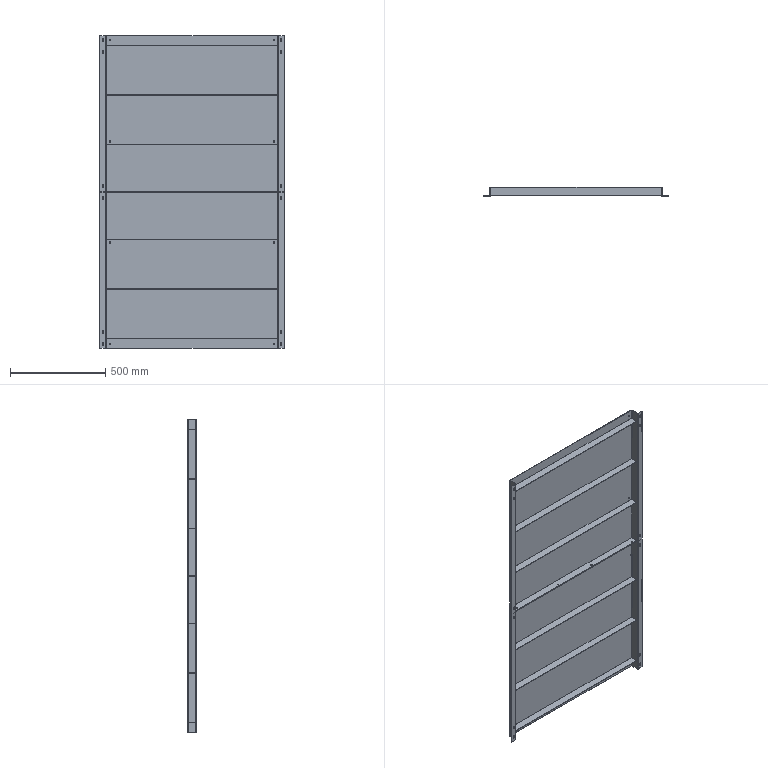Part | SolidWorks | 10 solids | 200 faces | box 966 x 49 x 1640 mm | volume 6033674 mm3 | cylinder 100 | plane 100 | commonest cylinder face diameters 9 x36 7 x32 4 x24 10 x8